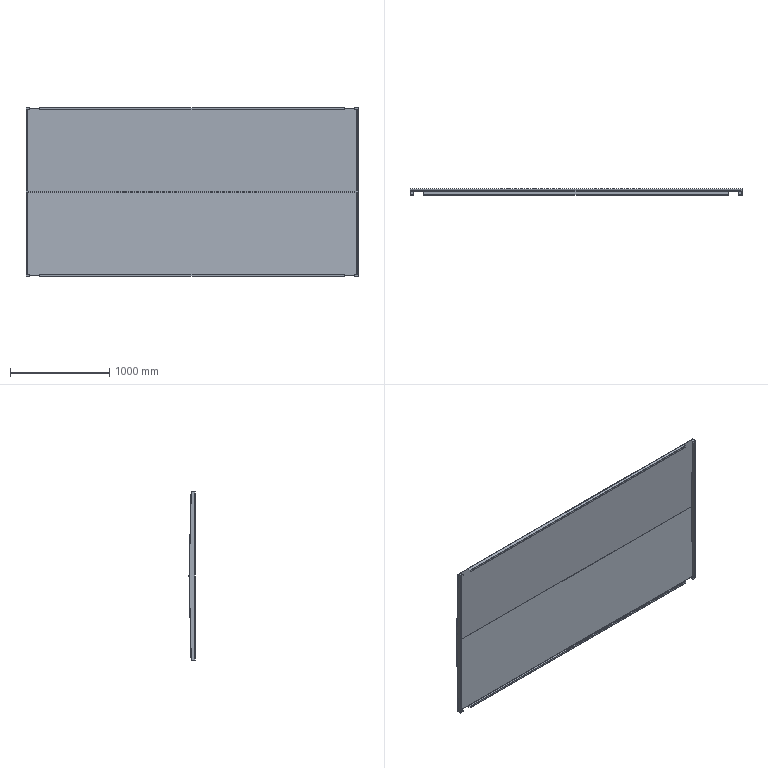Part | SolidWorks | 3 solids | 164 faces | box 3340 x 60.858 x 1696 mm | volume 15514481 mm3 | plane 130 | cylinder 34 | commonest cylinder face diameters 1 x10 0.2 x9 5.2 x9 6 x6